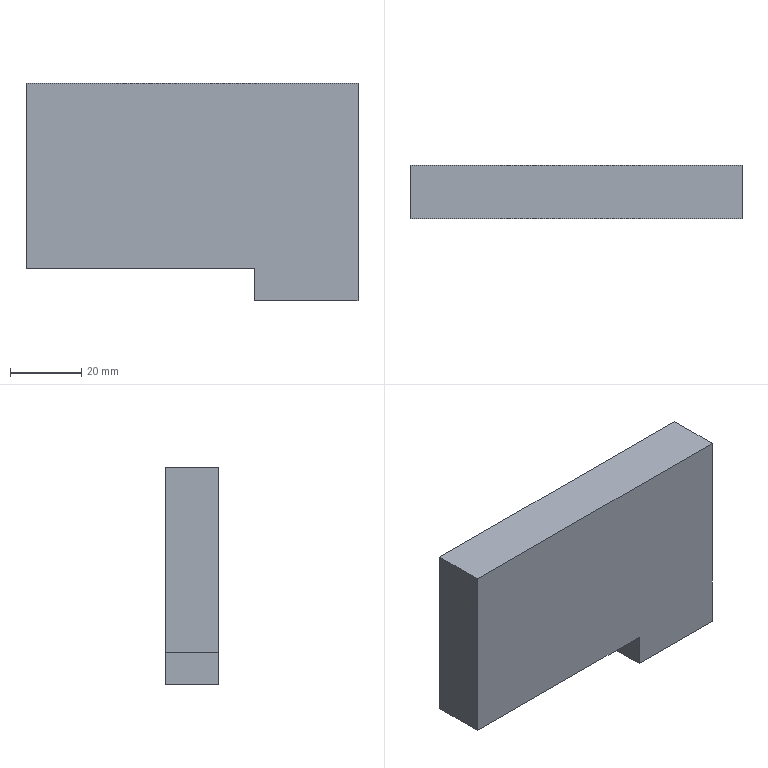Part | SolidWorks | features FlatPattern 1, SMBaseFlange 1, SheetMetal 1 | 1 solid | 8 faces | box 93 x 15 x 61 mm | volume 76455 mm3 | plane 8
STEP:
#1=CARTESIAN_POINT('',(64.,0.,0.));
#2=VERTEX_POINT('',#1);
#3=CARTESIAN_POINT('',(0.,0.,0.));
#4=VERTEX_POINT('',#3);
#5=CARTESIAN_POINT('',(64.,0.,0.));
#6=DIRECTION('',(-1.,0.,0.));
#7=VECTOR('',#6,1000.);
#8=LINE('',#5,#7);
#9=EDGE_CURVE('',#2,#4,#8,.T.);
#10=ORIENTED_EDGE('',*,*,#9,.F.);
#11=CARTESIAN_POINT('',(64.,-15.,0.));
#12=VERTEX_POINT('',#11);
#13=CARTESIAN_POINT('',(64.,-15.,0.));
#14=DIRECTION('',(0.,1.,0.));
#15=VECTOR('',#14,1000.);
#16=LINE('',#13,#15);
#17=EDGE_CURVE('',#12,#2,#16,.T.);
#18=ORIENTED_EDGE('',*,*,#17,.F.);
#19=CARTESIAN_POINT('',(0.,-15.,0.));
#20=VERTEX_POINT('',#19);
#21=CARTESIAN_POINT('',(64.,-15.,0.));
#22=DIRECTION('',(-1.,0.,0.));
#23=VECTOR('',#22,1000.);
#24=LINE('',#21,#23);
#25=EDGE_CURVE('',#12,#20,#24,.T.);
#26=ORIENTED_EDGE('',*,*,#25,.T.);
#27=CARTESIAN_POINT('',(0.,-15.,0.));
#28=DIRECTION('',(0.,1.,0.));
#29=VECTOR('',#28,1000.);
#30=LINE('',#27,#29);
#31=EDGE_CURVE('',#20,#4,#30,.T.);
#32=ORIENTED_EDGE('',*,*,#31,.T.);
#33=EDGE_LOOP('',(#10,#18,#26,#32));
#34=FACE_OUTER_BOUND('',#33,.T.);
#35=CARTESIAN_POINT('',(64.,-15.,0.));
#36=DIRECTION('',(0.,0.,-1.));
#37=DIRECTION('',(-1.,0.,0.));
#38=AXIS2_PLACEMENT_3D('',#35,#36,#37);
#39=PLANE('',#38);
#40=ADVANCED_FACE('',(#34),#39,.T.);
#41=CARTESIAN_POINT('',(64.,0.,-9.));
#42=VERTEX_POINT('',#41);
#43=CARTESIAN_POINT('',(64.,0.,-9.));
#44=DIRECTION('',(0.,0.,1.));
#45=VECTOR('',#44,1000.);
#46=LINE('',#43,#45);
#47=EDGE_CURVE('',#42,#2,#46,.T.);
#48=ORIENTED_EDGE('',*,*,#47,.F.);
#49=CARTESIAN_POINT('',(64.,-15.,-9.));
#50=VERTEX_POINT('',#49);
#51=CARTESIAN_POINT('',(64.,-15.,-9.));
#52=DIRECTION('',(0.,1.,0.));
#53=VECTOR('',#52,1000.);
#54=LINE('',#51,#53);
#55=EDGE_CURVE('',#50,#42,#54,.T.);
#56=ORIENTED_EDGE('',*,*,#55,.F.);
#57=CARTESIAN_POINT('',(64.,-15.,-9.));
#58=DIRECTION('',(0.,0.,1.));
#59=VECTOR('',#58,1000.);
#60=LINE('',#57,#59);
#61=EDGE_CURVE('',#50,#12,#60,.T.);
#62=ORIENTED_EDGE('',*,*,#61,.T.);
#63=ORIENTED_EDGE('',*,*,#17,.T.);
#64=EDGE_LOOP('',(#48,#56,#62,#63));
#65=FACE_OUTER_BOUND('',#64,.T.);
#66=CARTESIAN_POINT('',(64.,-15.,-9.));
#67=DIRECTION('',(-1.,0.,0.));
#68=DIRECTION('',(0.,0.,1.));
#69=AXIS2_PLACEMENT_3D('',#66,#67,#68);
#70=PLANE('',#69);
#71=ADVANCED_FACE('',(#65),#70,.T.);
#72=CARTESIAN_POINT('',(93.,0.,-9.));
#73=VERTEX_POINT('',#72);
#74=CARTESIAN_POINT('',(93.,0.,-9.));
#75=DIRECTION('',(-1.,0.,0.));
#76=VECTOR('',#75,1000.);
#77=LINE('',#74,#76);
#78=EDGE_CURVE('',#73,#42,#77,.T.);
#79=ORIENTED_EDGE('',*,*,#78,.F.);
#80=CARTESIAN_POINT('',(93.,-15.,-9.));
#81=VERTEX_POINT('',#80);
#82=CARTESIAN_POINT('',(93.,-15.,-9.));
#83=DIRECTION('',(0.,1.,0.));
#84=VECTOR('',#83,1000.);
#85=LINE('',#82,#84);
#86=EDGE_CURVE('',#81,#73,#85,.T.);
#87=ORIENTED_EDGE('',*,*,#86,.F.);
#88=CARTESIAN_POINT('',(93.,-15.,-9.));
#89=DIRECTION('',(-1.,0.,0.));
#90=VECTOR('',#89,1000.);
#91=LINE('',#88,#90);
#92=EDGE_CURVE('',#81,#50,#91,.T.);
#93=ORIENTED_EDGE('',*,*,#92,.T.);
#94=ORIENTED_EDGE('',*,*,#55,.T.);
#95=EDGE_LOOP('',(#79,#87,#93,#94));
#96=FACE_OUTER_BOUND('',#95,.T.);
#97=CARTESIAN_POINT('',(93.,-15.,-9.));
#98=DIRECTION('',(0.,0.,-1.));
#99=DIRECTION('',(-1.,0.,0.));
#100=AXIS2_PLACEMENT_3D('',#97,#98,#99);
#101=PLANE('',#100);
#102=ADVANCED_FACE('',(#96),#101,.T.);
#103=CARTESIAN_POINT('',(93.,0.,52.));
#104=VERTEX_POINT('',#103);
#105=CARTESIAN_POINT('',(93.,0.,52.));
#106=DIRECTION('',(0.,0.,-1.));
#107=VECTOR('',#106,1000.);
#108=LINE('',#105,#107);
#109=EDGE_CURVE('',#104,#73,#108,.T.);
#110=ORIENTED_EDGE('',*,*,#109,.F.);
#111=CARTESIAN_POINT('',(93.,-15.,52.));
#112=VERTEX_POINT('',#111);
#113=CARTESIAN_POINT('',(93.,-15.,52.));
#114=DIRECTION('',(0.,1.,0.));
#115=VECTOR('',#114,1000.);
#116=LINE('',#113,#115);
#117=EDGE_CURVE('',#112,#104,#116,.T.);
#118=ORIENTED_EDGE('',*,*,#117,.F.);
#119=CARTESIAN_POINT('',(93.,-15.,52.));
#120=DIRECTION('',(0.,0.,-1.));
#121=VECTOR('',#120,1000.);
#122=LINE('',#119,#121);
#123=EDGE_CURVE('',#112,#81,#122,.T.);
#124=ORIENTED_EDGE('',*,*,#123,.T.);
#125=ORIENTED_EDGE('',*,*,#86,.T.);
#126=EDGE_LOOP('',(#110,#118,#124,#125));
#127=FACE_OUTER_BOUND('',#126,.T.);
#128=CARTESIAN_POINT('',(93.,-15.,52.));
#129=DIRECTION('',(1.,0.,0.));
#130=DIRECTION('',(0.,0.,-1.));
#131=AXIS2_PLACEMENT_3D('',#128,#129,#130);
#132=PLANE('',#131);
#133=ADVANCED_FACE('',(#127),#132,.T.);
#134=CARTESIAN_POINT('',(0.,0.,52.));
#135=VERTEX_POINT('',#134);
#136=CARTESIAN_POINT('',(0.,0.,52.));
#137=DIRECTION('',(1.,0.,0.));
#138=VECTOR('',#137,1000.);
#139=LINE('',#136,#138);
#140=EDGE_CURVE('',#135,#104,#139,.T.);
#141=ORIENTED_EDGE('',*,*,#140,.F.);
#142=CARTESIAN_POINT('',(0.,-15.,52.));
#143=VERTEX_POINT('',#142);
#144=CARTESIAN_POINT('',(0.,-15.,52.));
#145=DIRECTION('',(0.,1.,0.));
#146=VECTOR('',#145,1000.);
#147=LINE('',#144,#146);
#148=EDGE_CURVE('',#143,#135,#147,.T.);
#149=ORIENTED_EDGE('',*,*,#148,.F.);
#150=CARTESIAN_POINT('',(0.,-15.,52.));
#151=DIRECTION('',(1.,0.,0.));
#152=VECTOR('',#151,1000.);
#153=LINE('',#150,#152);
#154=EDGE_CURVE('',#143,#112,#153,.T.);
#155=ORIENTED_EDGE('',*,*,#154,.T.);
#156=ORIENTED_EDGE('',*,*,#117,.T.);
#157=EDGE_LOOP('',(#141,#149,#155,#156));
#158=FACE_OUTER_BOUND('',#157,.T.);
#159=CARTESIAN_POINT('',(0.,-15.,52.));
#160=DIRECTION('',(0.,0.,1.));
#161=DIRECTION('',(1.,0.,0.));
#162=AXIS2_PLACEMENT_3D('',#159,#160,#161);
#163=PLANE('',#162);
#164=ADVANCED_FACE('',(#158),#163,.T.);
#165=CARTESIAN_POINT('',(0.,0.,0.));
#166=DIRECTION('',(0.,0.,1.));
#167=VECTOR('',#166,1000.);
#168=LINE('',#165,#167);
#169=EDGE_CURVE('',#4,#135,#168,.T.);
#170=ORIENTED_EDGE('',*,*,#169,.F.);
#171=ORIENTED_EDGE('',*,*,#31,.F.);
#172=CARTESIAN_POINT('',(0.,-15.,0.));
#173=DIRECTION('',(0.,0.,1.));
#174=VECTOR('',#173,1000.);
#175=LINE('',#172,#174);
#176=EDGE_CURVE('',#20,#143,#175,.T.);
#177=ORIENTED_EDGE('',*,*,#176,.T.);
#178=ORIENTED_EDGE('',*,*,#148,.T.);
#179=EDGE_LOOP('',(#170,#171,#177,#178));
#180=FACE_OUTER_BOUND('',#179,.T.);
#181=CARTESIAN_POINT('',(0.,-15.,0.));
#182=DIRECTION('',(-1.,0.,0.));
#183=DIRECTION('',(0.,0.,1.));
#184=AXIS2_PLACEMENT_3D('',#181,#182,#183);
#185=PLANE('',#184);
#186=ADVANCED_FACE('',(#180),#185,.T.);
#187=ORIENTED_EDGE('',*,*,#25,.F.);
#188=ORIENTED_EDGE('',*,*,#61,.F.);
#189=ORIENTED_EDGE('',*,*,#92,.F.);
#190=ORIENTED_EDGE('',*,*,#123,.F.);
#191=ORIENTED_EDGE('',*,*,#154,.F.);
#192=ORIENTED_EDGE('',*,*,#176,.F.);
#193=EDGE_LOOP('',(#187,#188,#189,#190,#191,#192));
#194=FACE_OUTER_BOUND('',#193,.T.);
#195=CARTESIAN_POINT('',(0.,-15.,0.));
#196=DIRECTION('',(0.,1.,0.));
#197=DIRECTION('',(0.,0.,1.));
#198=AXIS2_PLACEMENT_3D('',#195,#196,#197);
#199=PLANE('',#198);
#200=ADVANCED_FACE('',(#194),#199,.F.);
#201=ORIENTED_EDGE('',*,*,#9,.T.);
#202=ORIENTED_EDGE('',*,*,#169,.T.);
#203=ORIENTED_EDGE('',*,*,#140,.T.);
#204=ORIENTED_EDGE('',*,*,#109,.T.);
#205=ORIENTED_EDGE('',*,*,#78,.T.);
#206=ORIENTED_EDGE('',*,*,#47,.T.);
#207=EDGE_LOOP('',(#201,#202,#203,#204,#205,#206));
#208=FACE_OUTER_BOUND('',#207,.T.);
#209=CARTESIAN_POINT('',(0.,0.,0.));
#210=DIRECTION('',(0.,1.,0.));
#211=DIRECTION('',(0.,0.,1.));
#212=AXIS2_PLACEMENT_3D('',#209,#210,#211);
#213=PLANE('',#212);
#214=ADVANCED_FACE('',(#208),#213,.T.);
#215=CLOSED_SHELL('',(#40,#71,#102,#133,#164,#186,#200,#214));
#216=MANIFOLD_SOLID_BREP('',#215);
#217=CARTESIAN_POINT('',(0.,0.,0.));
#218=DIRECTION('',(0.,0.,1.));
#219=DIRECTION('',(1.,0.,0.));
#220=AXIS2_PLACEMENT_3D('',#217,#218,#219);
#221=(LENGTH_UNIT()NAMED_UNIT(*)SI_UNIT(.MILLI.,.METRE.));
#222=UNCERTAINTY_MEASURE_WITH_UNIT(LENGTH_MEASURE(0.00001),#221,'','');
#223=(NAMED_UNIT(*)PLANE_ANGLE_UNIT()SI_UNIT($,.RADIAN.));
#224=(NAMED_UNIT(*)SI_UNIT($,.STERADIAN.)SOLID_ANGLE_UNIT());
#225=(GEOMETRIC_REPRESENTATION_CONTEXT(3)GLOBAL_UNCERTAINTY_ASSIGNED_CONTEXT((#222))GLOBAL_UNIT_ASSIGNED_CONTEXT((#221,#223,#224))REPRESENTATION_CONTEXT('',''));
#226=ADVANCED_BREP_SHAPE_REPRESENTATION('',(#216,#220),#225);